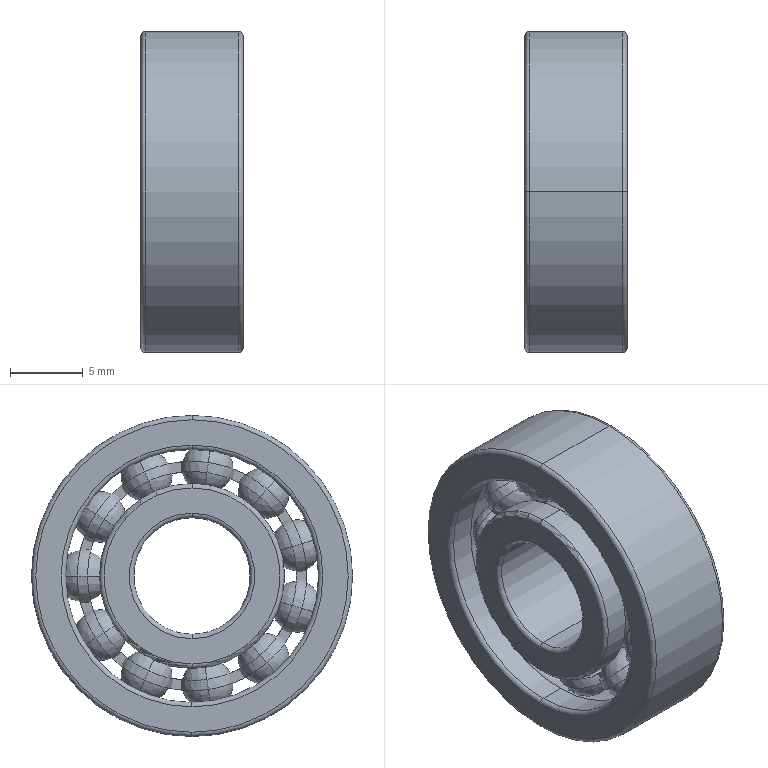Part | SolidWorks | features Revolution 4, CirPattern 2, RefAxis 1, RevCut 1 | 13 solids | 150 faces | box 7 x 22 x 22 mm | volume 1715 mm3 | cylinder 54 | sphere 48 | plane 26 | torus 22 | commonest cylinder face diameters 14.3 x21 15.7 x21 12.667 x4 17.333 x4 8 x2 22 x2